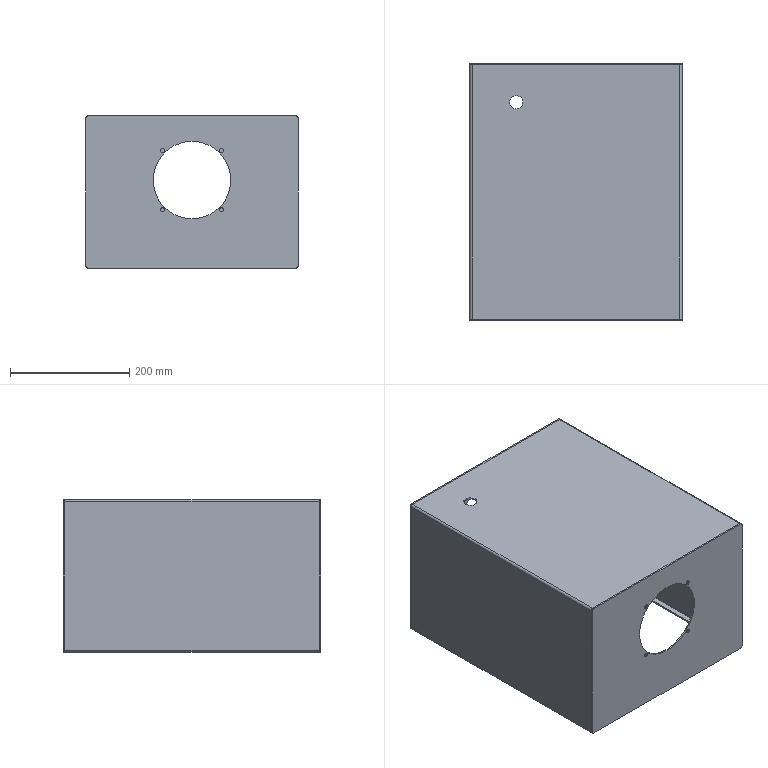Part | SolidWorks | features BaseBody 3 | 3 solids | 72 faces | box 355 x 431.16 x 255 mm | volume 1318329 mm3 | plane 42 | cylinder 30 | commonest cylinder face diameters 7 x12 6.8 x8 2 x4 130 x4 22 x2